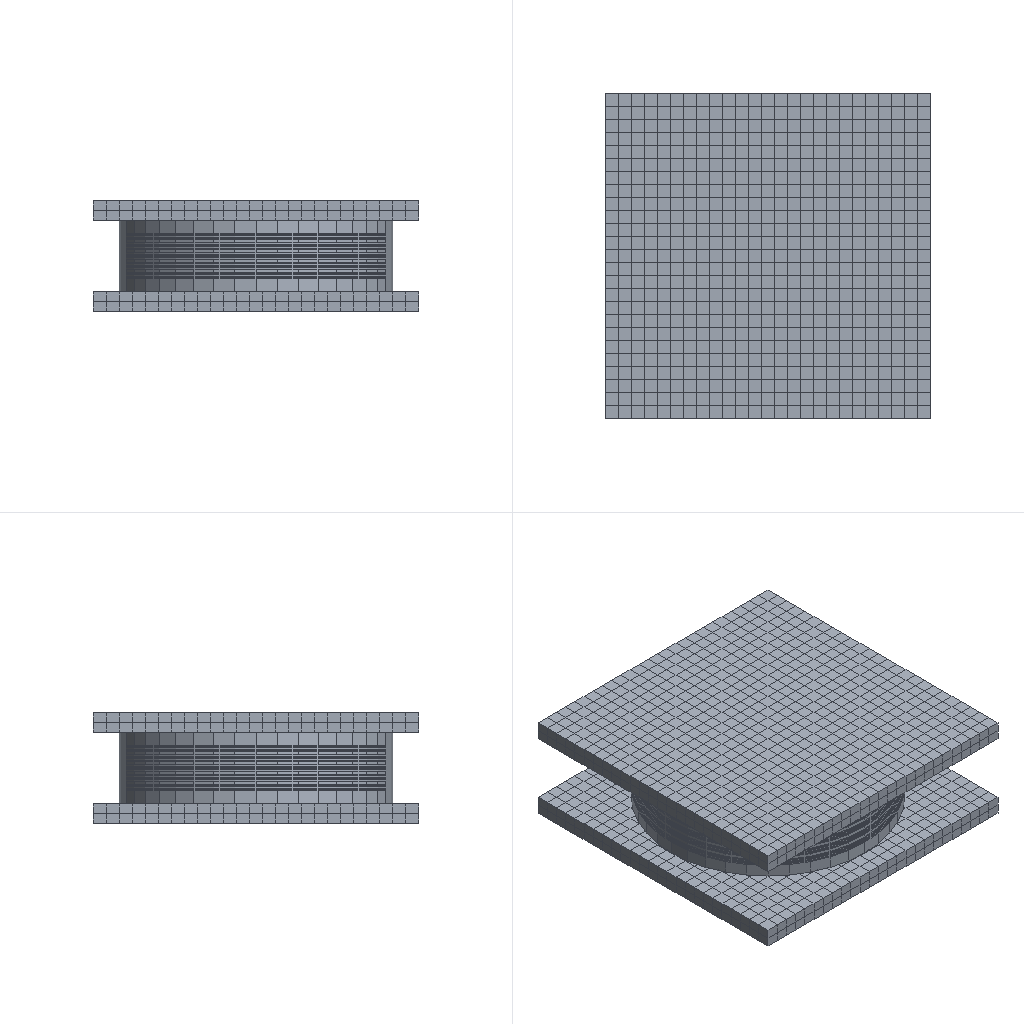Simulation study | abaqus
Set-up summary:
category,name,step,type,value,unit,region
solver,abaqus
solver,version,,,Abaqus/Standard 2020
units,not stated in the deck,,not stated
analysis,deck,,static,static
load_step,Step-1,Step-1,static
load_step,Step-2,Step-2,static
load_step,requested,,,2
mesh,nodes,,,10456
mesh,elements,,,7460
element_type,C3D8R,,solid,7460
load,load commands in deck,,count,3
bc,support commands in deck,,count,2
material,RUBBER,,in results
material,STEEL,,in results
check,setup vs results,,match,"per instance, exact: element labels, types and connectivity; labels of the nodes the elements use; coordinates of those nodes at SINGLE_PRECISION in 2 of 3 instance(s)"
Abaqus input file, long lists of numbers shortened:
*Heading
** Job name: Job-1 Model name: 10mm-5-shuiping-150-test7
** Generated by: Abaqus/CAE 2020
*Preprint, echo=NO, model=NO, history=NO, contact=NO
**
** PARTS
**
*Part, name=gaiban
*Node
      1,        -250.,        -250.,          30.
      2,        -250.,        -230.,          30.
** (2026 more lines like these left out)
*Element, type=C3D8R
   1,   79,   80,  106,  105,    1,    2,   28,   27
   2,   80,   81,  107,  106,    2,    3,   29,   28
** (1248 more lines like these left out)
*Nset, nset=_PickedSet2, internal, generate
    1,  2028,     1
*Elset, elset=_PickedSet2, internal, generate
    1,  1250,     1
** Section: steel
*Solid Section, elset=_PickedSet2, material=steel
,
*End Part
**
*Part, name=zhuti
*Node
      1,        -210.,           0.,          90.
      2,           0.,         210.,          90.
** (6398 more lines like these left out)
*Element, type=C3D8R
  1,  152, 1361, 4241, 1337,    1,   97, 1265,  122
  2, 1361, 1362, 4242, 4241,   97,   98, 1266, 1265
** (4958 more lines like these left out)
*Nset, nset=_PickedSet25, internal
    1,    2,    3,    4,    5,    6,    7,    8,    9,   10,   11,   12,   13,   14,   15,   16
   17,   18,   19,   20,   21,   22,   23,   24,   25,   26,   27,   28,   29,   30,   31,   32
** (148 more lines like these left out)
*Elset, elset=_PickedSet25, internal
  801,  802,  803,  804,  805,  806,  807,  808,  809,  810,  811,  812,  813,  814,  815,  816
  817,  818,  819,  820,  821,  822,  823,  824,  825,  826,  827,  828,  829,  830,  831,  832
** (58 more lines like these left out)
*Nset, nset=_PickedSet26, internal
    1,    2,    3,    4,    5,    6,    7,    8,    9,   10,   11,   12,   13,   14,   15,   16
   17,   18,   19,   20,   21,   22,   23,   24,   25,   26,   27,   28,   29,   30,   31,   32
** (373 more lines like these left out)
*Elset, elset=_PickedSet26, internal
    1,    2,    3,    4,    5,    6,    7,    8,    9,   10,   11,   12,   13,   14,   15,   16
   17,   18,   19,   20,   21,   22,   23,   24,   25,   26,   27,   28,   29,   30,   31,   32
** (248 more lines like these left out)
** Section: rubber
*Solid Section, elset=_PickedSet26, material=rubber
,
** Section: steel
*Solid Section, elset=_PickedSet25, material=steel
,
*End Part
**
**
** ASSEMBLY
**
*Assembly, name=Assembly
**
*Instance, name=gaiban-1, part=gaiban
*End Instance
**
*Instance, name=zhuti-1, part=zhuti
          0.,           0.,          30.
*End Instance
**
*Instance, name=gaiban-2, part=gaiban
          0.,           0.,         140.
*End Instance
**
*Node
      1,           0.,           0.,         170.
*Nset, nset=m_Set-1
 1,
*Nset, nset=_PickedSet16, internal, instance=gaiban-1
   53,   54,   55,   56,   57,   58,   59,   60,   61,   62,   63,   64,   65,   66,   67,   68
   69,   70,   71,   72,   73,   74,   75,   76,   77,   78,  131,  132,  133,  134,  135,  136
** (41 more lines like these left out)
*Elset, elset=_PickedSet16, internal, instance=gaiban-1
   26,   27,   28,   29,   30,   31,   32,   33,   34,   35,   36,   37,   38,   39,   40,   41
   42,   43,   44,   45,   46,   47,   48,   49,   50,   76,   77,   78,   79,   80,   81,   82
** (38 more lines like these left out)
*Nset, nset=_PickedSet17, internal
 1,
*Elset, elset=__PickedSurf11_S5, internal, instance=gaiban-2
   26,   27,   28,   29,   30,   31,   32,   33,   34,   35,   36,   37,   38,   39,   40,   41
   42,   43,   44,   45,   46,   47,   48,   49,   50,   76,   77,   78,   79,   80,   81,   82
** (38 more lines like these left out)
*Surface, type=ELEMENT, name=_PickedSurf11, internal
__PickedSurf11_S5, S5
*Elset, elset=__PickedSurf12_S2, internal, instance=zhuti-1, generate
 4801,  4960,     1
*Surface, type=ELEMENT, name=_PickedSurf12, internal
__PickedSurf12_S2, S2
*Elset, elset=__PickedSurf13_S3, internal, instance=gaiban-1
    1,    2,    3,    4,    5,    6,    7,    8,    9,   10,   11,   12,   13,   14,   15,   16
   17,   18,   19,   20,   21,   22,   23,   24,   25,   51,   52,   53,   54,   55,   56,   57
** (38 more lines like these left out)
*Surface, type=ELEMENT, name=_PickedSurf13, internal
__PickedSurf13_S3, S3
*Elset, elset=__PickedSurf14_S5, internal, instance=zhuti-1, generate
 4641,  4800,     1
*Surface, type=ELEMENT, name=_PickedSurf14, internal
__PickedSurf14_S5, S5
*Elset, elset=__PickedSurf15_S3, internal, instance=gaiban-2
    1,    2,    3,    4,    5,    6,    7,    8,    9,   10,   11,   12,   13,   14,   15,   16
   17,   18,   19,   20,   21,   22,   23,   24,   25,   51,   52,   53,   54,   55,   56,   57
** (38 more lines like these left out)
*Surface, type=ELEMENT, name=_PickedSurf15, internal
__PickedSurf15_S3, S3
*Elset, elset=__PickedSurf19_S3, internal, instance=gaiban-2
    1,    2,    3,    4,    5,    6,    7,    8,    9,   10,   11,   12,   13,   14,   15,   16
   17,   18,   19,   20,   21,   22,   23,   24,   25,   51,   52,   53,   54,   55,   56,   57
** (38 more lines like these left out)
*Surface, type=ELEMENT, name=_PickedSurf19, internal
__PickedSurf19_S3, S3
** Constraint: Constraint-1
*Coupling, constraint name=Constraint-1, ref node=m_Set-1, surface=_PickedSurf19
*Kinematic
** Constraint: Constraint-2
*Tie, name=Constraint-2, adjust=yes
_PickedSurf12, _PickedSurf11
** Constraint: Constraint-3
*Tie, name=Constraint-3, adjust=yes
_PickedSurf14, _PickedSurf13
*Spring, elset=Springs/Dashpots-1-spring
1
7000.
*Dashpot, elset=Springs/Dashpots-1-dashpot
1
7000.
*Element, type=Spring1, elset=Springs/Dashpots-1-spring
1, 1
*Element, type=Dashpot1, elset=Springs/Dashpots-1-dashpot
2, 1
*End Assembly
*Amplitude, name=Amp-1
             0.,              0.,              1.,             15.,              2.,              0.,              3.,            -15.
             4.,              0.,              5.,             20.,              6.,              0.,              7.,            -20.
             8.,              0.,              9.,             25.,             10.,              0.,             11.,            -25.
            12.,              0.,             13.,             30.,             14.,              0.,             15.,            -30.
            16.,              0.
**
** MATERIALS
**
*Material, name=rubber
*Density
 1.3e-09,
*Elastic
15., 0.4
*Plastic
 5.,    0.
 8., 0.003
10.,  0.01
*Material, name=steel
*Density
 7.8e-09,
*Elastic
206000., 0.3
**
** BOUNDARY CONDITIONS
**
** Name: BC-1 Type: 对称/反对称/完全固定
*Boundary
_PickedSet16, ENCASTRE
** ----------------------------------------------------------------
**
** STEP: Step-1
**
*Step, name=Step-1, nlgeom=YES
*Static
0.01, 1., 1e-05, 1.
**
** LOADS
**
** Name: Load-1   Type: Pressure
*Dsload
_PickedSurf15, P, 0.5
**
** OUTPUT REQUESTS
**
*Restart, write, number interval=1, time marks=NO
**
** FIELD OUTPUT: F-Output-1
**
*Output, field, variable=PRESELECT
*Output, history, frequency=0
*End Step
** ----------------------------------------------------------------
**
** STEP: Step-2
**
*Step, name=Step-2, nlgeom=YES, inc=1000
*Static, stabilize=0.0002, allsdtol=0.05, continue=NO
0.01, 16., 1.6e-05, 16.
**
** BOUNDARY CONDITIONS
**
** Name: BC-2 Type: 位移/转角
*Boundary, amplitude=Amp-1
_PickedSet17, 1, 1, 1.
**
** LOADS
**
** Name: Load-1   Type: Pressure
*Dsload
_PickedSurf15, P, 0.5
**
** OUTPUT REQUESTS
**
*Restart, write, number interval=1, time marks=NO
**
** FIELD OUTPUT: F-Output-1
**
*Output, field
*Node Output
CF, RF, U, V
*Element Output, directions=YES
E, LE, MISES, MISESMAX, PE, PEEQ, PEMAG, S
*Contact Output
CDISP, CSTRESS
**
** HISTORY OUTPUT: H-Output-1
**
*Output, history
*Node Output, nset=m_Set-1
RF1, U1
*End Step
Results summary:
result,step,,completed,increments=11 time=1.0/1.0
result,step,,partial,increments=102 time=10.89/16.0
result,analysis,,,static
result,last_loadstep,,,2
result,primary field,,,U
result,reaction total,,FX,-336805.714,model units
result,reaction total,,FY,0.0,model units
result,reaction total,,FZ,124859.45,model units